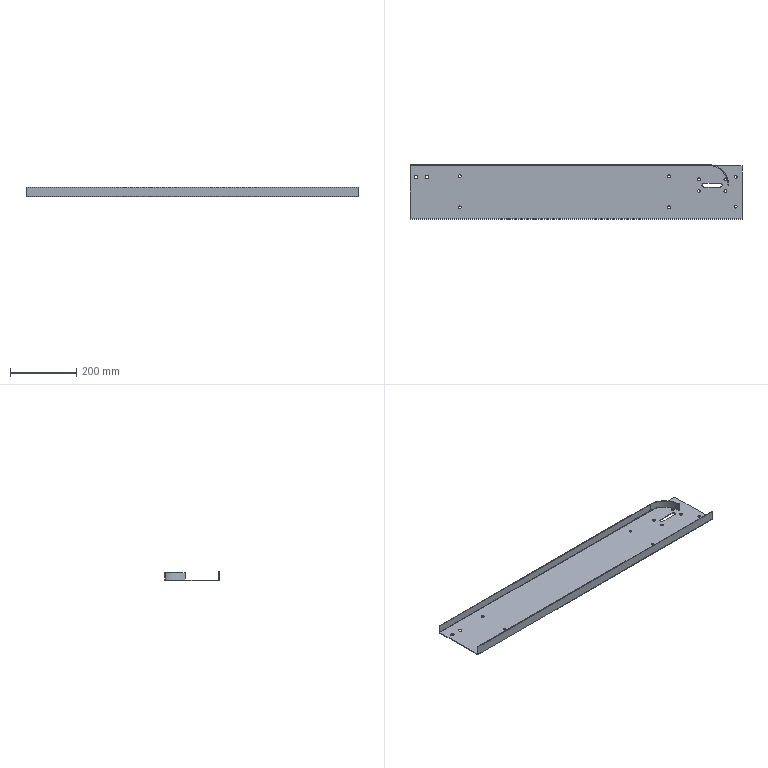Part | SolidWorks | features BaseBody 1 | 1 solid | 50 faces | box 1000 x 165 x 30 mm | volume 425735 mm3 | cylinder 33 | plane 16 | spline 1 | commonest cylinder face diameters 8.5 x20 11 x7 1.473 x2 5.473 x2 120 x1 124 x1